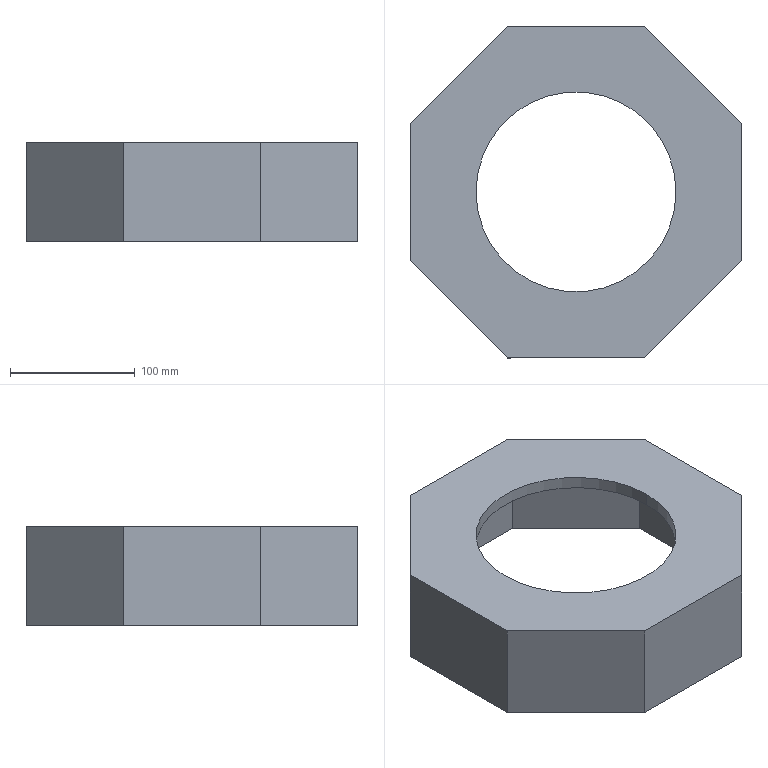Part | SolidWorks | features Cut 1, Extrusion 1, Shell 1 | 1 solid | 21 faces | box 265.563 x 265.563 x 80 mm | volume 975982 mm3 | plane 19 | cylinder 2 | commonest cylinder face diameters 160 x2
STEP:
#1=CARTESIAN_POINT('',(-679.884,-90.,70.));
#2=VERTEX_POINT('',#1);
#3=CARTESIAN_POINT('',(-519.884,-90.,70.));
#4=VERTEX_POINT('',#3);
#5=CARTESIAN_POINT('',(-599.884,-90.,70.));
#6=DIRECTION('',(0.,0.,1.));
#7=DIRECTION('',(1.,0.,0.));
#8=AXIS2_PLACEMENT_3D('',#5,#6,#7);
#9=CIRCLE('',#8,80.);
#10=EDGE_CURVE('',#2,#4,#9,.T.);
#11=ORIENTED_EDGE('',*,*,#10,.F.);
#12=CARTESIAN_POINT('',(-679.884,-90.,80.));
#13=VERTEX_POINT('',#12);
#14=CARTESIAN_POINT('',(-679.884,-90.,0.));
#15=DIRECTION('',(0.,0.,1.));
#16=VECTOR('',#15,1000.);
#17=LINE('',#14,#16);
#18=EDGE_CURVE('',#2,#13,#17,.T.);
#19=ORIENTED_EDGE('',*,*,#18,.T.);
#20=CARTESIAN_POINT('',(-519.884,-90.,80.));
#21=VERTEX_POINT('',#20);
#22=CARTESIAN_POINT('',(-599.884,-90.,80.));
#23=DIRECTION('',(0.,0.,1.));
#24=DIRECTION('',(1.,0.,0.));
#25=AXIS2_PLACEMENT_3D('',#22,#23,#24);
#26=CIRCLE('',#25,80.);
#27=EDGE_CURVE('',#13,#21,#26,.T.);
#28=ORIENTED_EDGE('',*,*,#27,.T.);
#29=CARTESIAN_POINT('',(-519.884,-90.,0.));
#30=DIRECTION('',(0.,0.,1.));
#31=VECTOR('',#30,1000.);
#32=LINE('',#29,#31);
#33=EDGE_CURVE('',#4,#21,#32,.T.);
#34=ORIENTED_EDGE('',*,*,#33,.F.);
#35=EDGE_LOOP('',(#11,#19,#28,#34));
#36=FACE_OUTER_BOUND('',#35,.T.);
#37=CARTESIAN_POINT('',(-599.884,-90.,0.));
#38=DIRECTION('',(0.,0.,1.));
#39=DIRECTION('',(1.,0.,0.));
#40=AXIS2_PLACEMENT_3D('',#37,#38,#39);
#41=CYLINDRICAL_SURFACE('',#40,80.);
#42=ADVANCED_FACE('',(#36),#41,.F.);
#43=CARTESIAN_POINT('',(-467.102,-145.,0.));
#44=VERTEX_POINT('',#43);
#45=CARTESIAN_POINT('',(-467.102,-35.,0.));
#46=VERTEX_POINT('',#45);
#47=CARTESIAN_POINT('',(-467.102,-145.,0.));
#48=DIRECTION('',(0.,1.,0.));
#49=VECTOR('',#48,1000.);
#50=LINE('',#47,#49);
#51=EDGE_CURVE('',#44,#46,#50,.T.);
#52=ORIENTED_EDGE('',*,*,#51,.T.);
#53=CARTESIAN_POINT('',(-467.102,-35.,80.));
#54=VERTEX_POINT('',#53);
#55=CARTESIAN_POINT('',(-467.102,-35.,80.));
#56=DIRECTION('',(0.,0.,-1.));
#57=VECTOR('',#56,1000.);
#58=LINE('',#55,#57);
#59=EDGE_CURVE('',#54,#46,#58,.T.);
#60=ORIENTED_EDGE('',*,*,#59,.F.);
#61=CARTESIAN_POINT('',(-467.102,-145.,80.));
#62=VERTEX_POINT('',#61);
#63=CARTESIAN_POINT('',(-467.102,-145.,80.));
#64=DIRECTION('',(0.,1.,0.));
#65=VECTOR('',#64,1000.);
#66=LINE('',#63,#65);
#67=EDGE_CURVE('',#62,#54,#66,.T.);
#68=ORIENTED_EDGE('',*,*,#67,.F.);
#69=CARTESIAN_POINT('',(-467.102,-145.,80.));
#70=DIRECTION('',(0.,0.,-1.));
#71=VECTOR('',#70,1000.);
#72=LINE('',#69,#71);
#73=EDGE_CURVE('',#62,#44,#72,.T.);
#74=ORIENTED_EDGE('',*,*,#73,.T.);
#75=EDGE_LOOP('',(#52,#60,#68,#74));
#76=FACE_OUTER_BOUND('',#75,.T.);
#77=CARTESIAN_POINT('',(-467.102,-145.,80.));
#78=DIRECTION('',(-1.,0.,0.));
#79=DIRECTION('',(0.,-1.,0.));
#80=AXIS2_PLACEMENT_3D('',#77,#78,#79);
#81=PLANE('',#80);
#82=ADVANCED_FACE('',(#76),#81,.F.);
#83=CARTESIAN_POINT('',(-544.884,42.782,0.));
#84=VERTEX_POINT('',#83);
#85=CARTESIAN_POINT('',(-467.102,-35.,0.));
#86=DIRECTION('',(-0.7071,0.7071,0.));
#87=VECTOR('',#86,1000.);
#88=LINE('',#85,#87);
#89=EDGE_CURVE('',#46,#84,#88,.T.);
#90=ORIENTED_EDGE('',*,*,#89,.T.);
#91=CARTESIAN_POINT('',(-544.884,42.782,80.));
#92=VERTEX_POINT('',#91);
#93=CARTESIAN_POINT('',(-544.884,42.782,80.));
#94=DIRECTION('',(0.,0.,-1.));
#95=VECTOR('',#94,1000.);
#96=LINE('',#93,#95);
#97=EDGE_CURVE('',#92,#84,#96,.T.);
#98=ORIENTED_EDGE('',*,*,#97,.F.);
#99=CARTESIAN_POINT('',(-467.102,-35.,80.));
#100=DIRECTION('',(-0.7071,0.7071,0.));
#101=VECTOR('',#100,1000.);
#102=LINE('',#99,#101);
#103=EDGE_CURVE('',#54,#92,#102,.T.);
#104=ORIENTED_EDGE('',*,*,#103,.F.);
#105=ORIENTED_EDGE('',*,*,#59,.T.);
#106=EDGE_LOOP('',(#90,#98,#104,#105));
#107=FACE_OUTER_BOUND('',#106,.T.);
#108=CARTESIAN_POINT('',(-467.102,-35.,80.));
#109=DIRECTION('',(-0.7071,-0.7071,0.));
#110=DIRECTION('',(0.7071,-0.7071,0.));
#111=AXIS2_PLACEMENT_3D('',#108,#109,#110);
#112=PLANE('',#111);
#113=ADVANCED_FACE('',(#107),#112,.F.);
#114=CARTESIAN_POINT('',(-654.884,42.782,0.));
#115=VERTEX_POINT('',#114);
#116=CARTESIAN_POINT('',(-544.884,42.782,0.));
#117=DIRECTION('',(-1.,0.,0.));
#118=VECTOR('',#117,1000.);
#119=LINE('',#116,#118);
#120=EDGE_CURVE('',#84,#115,#119,.T.);
#121=ORIENTED_EDGE('',*,*,#120,.T.);
#122=CARTESIAN_POINT('',(-654.884,42.782,80.));
#123=VERTEX_POINT('',#122);
#124=CARTESIAN_POINT('',(-654.884,42.782,80.));
#125=DIRECTION('',(0.,0.,-1.));
#126=VECTOR('',#125,1000.);
#127=LINE('',#124,#126);
#128=EDGE_CURVE('',#123,#115,#127,.T.);
#129=ORIENTED_EDGE('',*,*,#128,.F.);
#130=CARTESIAN_POINT('',(-544.884,42.782,80.));
#131=DIRECTION('',(-1.,0.,0.));
#132=VECTOR('',#131,1000.);
#133=LINE('',#130,#132);
#134=EDGE_CURVE('',#92,#123,#133,.T.);
#135=ORIENTED_EDGE('',*,*,#134,.F.);
#136=ORIENTED_EDGE('',*,*,#97,.T.);
#137=EDGE_LOOP('',(#121,#129,#135,#136));
#138=FACE_OUTER_BOUND('',#137,.T.);
#139=CARTESIAN_POINT('',(-544.884,42.782,80.));
#140=DIRECTION('',(0.,-1.,0.));
#141=DIRECTION('',(1.,0.,0.));
#142=AXIS2_PLACEMENT_3D('',#139,#140,#141);
#143=PLANE('',#142);
#144=ADVANCED_FACE('',(#138),#143,.F.);
#145=CARTESIAN_POINT('',(-732.666,-35.,0.));
#146=VERTEX_POINT('',#145);
#147=CARTESIAN_POINT('',(-654.884,42.782,0.));
#148=DIRECTION('',(-0.7071,-0.7071,0.));
#149=VECTOR('',#148,1000.);
#150=LINE('',#147,#149);
#151=EDGE_CURVE('',#115,#146,#150,.T.);
#152=ORIENTED_EDGE('',*,*,#151,.T.);
#153=CARTESIAN_POINT('',(-732.666,-35.,80.));
#154=VERTEX_POINT('',#153);
#155=CARTESIAN_POINT('',(-732.666,-35.,80.));
#156=DIRECTION('',(0.,0.,-1.));
#157=VECTOR('',#156,1000.);
#158=LINE('',#155,#157);
#159=EDGE_CURVE('',#154,#146,#158,.T.);
#160=ORIENTED_EDGE('',*,*,#159,.F.);
#161=CARTESIAN_POINT('',(-654.884,42.782,80.));
#162=DIRECTION('',(-0.7071,-0.7071,0.));
#163=VECTOR('',#162,1000.);
#164=LINE('',#161,#163);
#165=EDGE_CURVE('',#123,#154,#164,.T.);
#166=ORIENTED_EDGE('',*,*,#165,.F.);
#167=ORIENTED_EDGE('',*,*,#128,.T.);
#168=EDGE_LOOP('',(#152,#160,#166,#167));
#169=FACE_OUTER_BOUND('',#168,.T.);
#170=CARTESIAN_POINT('',(-654.884,42.782,80.));
#171=DIRECTION('',(0.7071,-0.7071,0.));
#172=DIRECTION('',(0.7071,0.7071,0.));
#173=AXIS2_PLACEMENT_3D('',#170,#171,#172);
#174=PLANE('',#173);
#175=ADVANCED_FACE('',(#169),#174,.F.);
#176=CARTESIAN_POINT('',(-732.666,-145.,0.));
#177=VERTEX_POINT('',#176);
#178=CARTESIAN_POINT('',(-732.666,-35.,0.));
#179=DIRECTION('',(0.,-1.,0.));
#180=VECTOR('',#179,1000.);
#181=LINE('',#178,#180);
#182=EDGE_CURVE('',#146,#177,#181,.T.);
#183=ORIENTED_EDGE('',*,*,#182,.T.);
#184=CARTESIAN_POINT('',(-732.666,-145.,80.));
#185=VERTEX_POINT('',#184);
#186=CARTESIAN_POINT('',(-732.666,-145.,80.));
#187=DIRECTION('',(0.,0.,-1.));
#188=VECTOR('',#187,1000.);
#189=LINE('',#186,#188);
#190=EDGE_CURVE('',#185,#177,#189,.T.);
#191=ORIENTED_EDGE('',*,*,#190,.F.);
#192=CARTESIAN_POINT('',(-732.666,-35.,80.));
#193=DIRECTION('',(0.,-1.,0.));
#194=VECTOR('',#193,1000.);
#195=LINE('',#192,#194);
#196=EDGE_CURVE('',#154,#185,#195,.T.);
#197=ORIENTED_EDGE('',*,*,#196,.F.);
#198=ORIENTED_EDGE('',*,*,#159,.T.);
#199=EDGE_LOOP('',(#183,#191,#197,#198));
#200=FACE_OUTER_BOUND('',#199,.T.);
#201=CARTESIAN_POINT('',(-732.666,-35.,80.));
#202=DIRECTION('',(1.,0.,0.));
#203=DIRECTION('',(0.,1.,0.));
#204=AXIS2_PLACEMENT_3D('',#201,#202,#203);
#205=PLANE('',#204);
#206=ADVANCED_FACE('',(#200),#205,.F.);
#207=CARTESIAN_POINT('',(-654.884,-222.782,0.));
#208=VERTEX_POINT('',#207);
#209=CARTESIAN_POINT('',(-732.666,-145.,0.));
#210=DIRECTION('',(0.7071,-0.7071,0.));
#211=VECTOR('',#210,1000.);
#212=LINE('',#209,#211);
#213=EDGE_CURVE('',#177,#208,#212,.T.);
#214=ORIENTED_EDGE('',*,*,#213,.T.);
#215=CARTESIAN_POINT('',(-654.884,-222.782,80.));
#216=VERTEX_POINT('',#215);
#217=CARTESIAN_POINT('',(-654.884,-222.782,80.));
#218=DIRECTION('',(0.,0.,-1.));
#219=VECTOR('',#218,1000.);
#220=LINE('',#217,#219);
#221=EDGE_CURVE('',#216,#208,#220,.T.);
#222=ORIENTED_EDGE('',*,*,#221,.F.);
#223=CARTESIAN_POINT('',(-732.666,-145.,80.));
#224=DIRECTION('',(0.7071,-0.7071,0.));
#225=VECTOR('',#224,1000.);
#226=LINE('',#223,#225);
#227=EDGE_CURVE('',#185,#216,#226,.T.);
#228=ORIENTED_EDGE('',*,*,#227,.F.);
#229=ORIENTED_EDGE('',*,*,#190,.T.);
#230=EDGE_LOOP('',(#214,#222,#228,#229));
#231=FACE_OUTER_BOUND('',#230,.T.);
#232=CARTESIAN_POINT('',(-732.666,-145.,80.));
#233=DIRECTION('',(0.7071,0.7071,0.));
#234=DIRECTION('',(-0.7071,0.7071,0.));
#235=AXIS2_PLACEMENT_3D('',#232,#233,#234);
#236=PLANE('',#235);
#237=ADVANCED_FACE('',(#231),#236,.F.);
#238=CARTESIAN_POINT('',(-544.884,-222.782,0.));
#239=VERTEX_POINT('',#238);
#240=CARTESIAN_POINT('',(-654.884,-222.782,0.));
#241=DIRECTION('',(1.,0.,0.));
#242=VECTOR('',#241,1000.);
#243=LINE('',#240,#242);
#244=EDGE_CURVE('',#208,#239,#243,.T.);
#245=ORIENTED_EDGE('',*,*,#244,.T.);
#246=CARTESIAN_POINT('',(-544.884,-222.782,80.));
#247=VERTEX_POINT('',#246);
#248=CARTESIAN_POINT('',(-544.884,-222.782,80.));
#249=DIRECTION('',(0.,0.,-1.));
#250=VECTOR('',#249,1000.);
#251=LINE('',#248,#250);
#252=EDGE_CURVE('',#247,#239,#251,.T.);
#253=ORIENTED_EDGE('',*,*,#252,.F.);
#254=CARTESIAN_POINT('',(-654.884,-222.782,80.));
#255=DIRECTION('',(1.,0.,0.));
#256=VECTOR('',#255,1000.);
#257=LINE('',#254,#256);
#258=EDGE_CURVE('',#216,#247,#257,.T.);
#259=ORIENTED_EDGE('',*,*,#258,.F.);
#260=ORIENTED_EDGE('',*,*,#221,.T.);
#261=EDGE_LOOP('',(#245,#253,#259,#260));
#262=FACE_OUTER_BOUND('',#261,.T.);
#263=CARTESIAN_POINT('',(-654.884,-222.782,80.));
#264=DIRECTION('',(0.,1.,0.));
#265=DIRECTION('',(-1.,0.,0.));
#266=AXIS2_PLACEMENT_3D('',#263,#264,#265);
#267=PLANE('',#266);
#268=ADVANCED_FACE('',(#262),#267,.F.);
#269=CARTESIAN_POINT('',(-544.884,-222.782,0.));
#270=DIRECTION('',(0.7071,0.7071,0.));
#271=VECTOR('',#270,1000.);
#272=LINE('',#269,#271);
#273=EDGE_CURVE('',#239,#44,#272,.T.);
#274=ORIENTED_EDGE('',*,*,#273,.T.);
#275=ORIENTED_EDGE('',*,*,#73,.F.);
#276=CARTESIAN_POINT('',(-544.884,-222.782,80.));
#277=DIRECTION('',(0.7071,0.7071,0.));
#278=VECTOR('',#277,1000.);
#279=LINE('',#276,#278);
#280=EDGE_CURVE('',#247,#62,#279,.T.);
#281=ORIENTED_EDGE('',*,*,#280,.F.);
#282=ORIENTED_EDGE('',*,*,#252,.T.);
#283=EDGE_LOOP('',(#274,#275,#281,#282));
#284=FACE_OUTER_BOUND('',#283,.T.);
#285=CARTESIAN_POINT('',(-544.884,-222.782,80.));
#286=DIRECTION('',(-0.7071,0.7071,0.));
#287=DIRECTION('',(-0.7071,-0.7071,0.));
#288=AXIS2_PLACEMENT_3D('',#285,#286,#287);
#289=PLANE('',#288);
#290=ADVANCED_FACE('',(#284),#289,.F.);
#291=CARTESIAN_POINT('',(-599.884,-90.,80.));
#292=DIRECTION('',(0.,0.,1.));
#293=DIRECTION('',(1.,0.,0.));
#294=AXIS2_PLACEMENT_3D('',#291,#292,#293);
#295=CIRCLE('',#294,80.);
#296=EDGE_CURVE('',#21,#13,#295,.T.);
#297=ORIENTED_EDGE('',*,*,#296,.F.);
#298=ORIENTED_EDGE('',*,*,#27,.F.);
#299=EDGE_LOOP('',(#297,#298));
#300=FACE_BOUND('',#299,.T.);
#301=ORIENTED_EDGE('',*,*,#67,.T.);
#302=ORIENTED_EDGE('',*,*,#103,.T.);
#303=ORIENTED_EDGE('',*,*,#134,.T.);
#304=ORIENTED_EDGE('',*,*,#165,.T.);
#305=ORIENTED_EDGE('',*,*,#196,.T.);
#306=ORIENTED_EDGE('',*,*,#227,.T.);
#307=ORIENTED_EDGE('',*,*,#258,.T.);
#308=ORIENTED_EDGE('',*,*,#280,.T.);
#309=EDGE_LOOP('',(#301,#302,#303,#304,#305,#306,#307,#308));
#310=FACE_OUTER_BOUND('',#309,.T.);
#311=CARTESIAN_POINT('',(0.,0.,80.));
#312=DIRECTION('',(0.,0.,1.));
#313=DIRECTION('',(1.,0.,0.));
#314=AXIS2_PLACEMENT_3D('',#311,#312,#313);
#315=PLANE('',#314);
#316=ADVANCED_FACE('',(#300,#310),#315,.T.);
#317=CARTESIAN_POINT('',(-549.026,-212.782,0.));
#318=VERTEX_POINT('',#317);
#319=CARTESIAN_POINT('',(-477.102,-140.858,0.));
#320=VERTEX_POINT('',#319);
#321=CARTESIAN_POINT('',(-551.955,-215.711,0.));
#322=DIRECTION('',(0.7071,0.7071,0.));
#323=VECTOR('',#322,1000.);
#324=LINE('',#321,#323);
#325=EDGE_CURVE('',#318,#320,#324,.T.);
#326=ORIENTED_EDGE('',*,*,#325,.T.);
#327=CARTESIAN_POINT('',(-477.102,-39.142,0.));
#328=VERTEX_POINT('',#327);
#329=CARTESIAN_POINT('',(-477.102,-145.,0.));
#330=DIRECTION('',(0.,1.,0.));
#331=VECTOR('',#330,1000.);
#332=LINE('',#329,#331);
#333=EDGE_CURVE('',#320,#328,#332,.T.);
#334=ORIENTED_EDGE('',*,*,#333,.T.);
#335=CARTESIAN_POINT('',(-549.026,32.782,0.));
#336=VERTEX_POINT('',#335);
#337=CARTESIAN_POINT('',(-474.174,-42.071,0.));
#338=DIRECTION('',(-0.7071,0.7071,0.));
#339=VECTOR('',#338,1000.);
#340=LINE('',#337,#339);
#341=EDGE_CURVE('',#328,#336,#340,.T.);
#342=ORIENTED_EDGE('',*,*,#341,.T.);
#343=CARTESIAN_POINT('',(-650.742,32.782,0.));
#344=VERTEX_POINT('',#343);
#345=CARTESIAN_POINT('',(-544.884,32.782,0.));
#346=DIRECTION('',(-1.,0.,0.));
#347=VECTOR('',#346,1000.);
#348=LINE('',#345,#347);
#349=EDGE_CURVE('',#336,#344,#348,.T.);
#350=ORIENTED_EDGE('',*,*,#349,.T.);
#351=CARTESIAN_POINT('',(-722.666,-39.142,0.));
#352=VERTEX_POINT('',#351);
#353=CARTESIAN_POINT('',(-647.813,35.711,0.));
#354=DIRECTION('',(-0.7071,-0.7071,0.));
#355=VECTOR('',#354,1000.);
#356=LINE('',#353,#355);
#357=EDGE_CURVE('',#344,#352,#356,.T.);
#358=ORIENTED_EDGE('',*,*,#357,.T.);
#359=CARTESIAN_POINT('',(-722.666,-140.858,0.));
#360=VERTEX_POINT('',#359);
#361=CARTESIAN_POINT('',(-722.666,-35.,0.));
#362=DIRECTION('',(0.,-1.,0.));
#363=VECTOR('',#362,1000.);
#364=LINE('',#361,#363);
#365=EDGE_CURVE('',#352,#360,#364,.T.);
#366=ORIENTED_EDGE('',*,*,#365,.T.);
#367=CARTESIAN_POINT('',(-650.742,-212.782,0.));
#368=VERTEX_POINT('',#367);
#369=CARTESIAN_POINT('',(-725.595,-137.929,0.));
#370=DIRECTION('',(0.7071,-0.7071,0.));
#371=VECTOR('',#370,1000.);
#372=LINE('',#369,#371);
#373=EDGE_CURVE('',#360,#368,#372,.T.);
#374=ORIENTED_EDGE('',*,*,#373,.T.);
#375=CARTESIAN_POINT('',(-654.884,-212.782,0.));
#376=DIRECTION('',(1.,0.,0.));
#377=VECTOR('',#376,1000.);
#378=LINE('',#375,#377);
#379=EDGE_CURVE('',#368,#318,#378,.T.);
#380=ORIENTED_EDGE('',*,*,#379,.T.);
#381=EDGE_LOOP('',(#326,#334,#342,#350,#358,#366,#374,#380));
#382=FACE_BOUND('',#381,.T.);
#383=ORIENTED_EDGE('',*,*,#51,.F.);
#384=ORIENTED_EDGE('',*,*,#273,.F.);
#385=ORIENTED_EDGE('',*,*,#244,.F.);
#386=ORIENTED_EDGE('',*,*,#213,.F.);
#387=ORIENTED_EDGE('',*,*,#182,.F.);
#388=ORIENTED_EDGE('',*,*,#151,.F.);
#389=ORIENTED_EDGE('',*,*,#120,.F.);
#390=ORIENTED_EDGE('',*,*,#89,.F.);
#391=EDGE_LOOP('',(#383,#384,#385,#386,#387,#388,#389,#390));
#392=FACE_OUTER_BOUND('',#391,.T.);
#393=CARTESIAN_POINT('',(0.,0.,0.));
#394=DIRECTION('',(0.,0.,1.));
#395=DIRECTION('',(1.,0.,0.));
#396=AXIS2_PLACEMENT_3D('',#393,#394,#395);
#397=PLANE('',#396);
#398=ADVANCED_FACE('',(#382,#392),#397,.F.);
#399=ORIENTED_EDGE('',*,*,#333,.F.);
#400=CARTESIAN_POINT('',(-477.102,-140.858,70.));
#401=VERTEX_POINT('',#400);
#402=CARTESIAN_POINT('',(-477.102,-140.858,80.));
#403=DIRECTION('',(0.,0.,-1.));
#404=VECTOR('',#403,1000.);
#405=LINE('',#402,#404);
#406=EDGE_CURVE('',#401,#320,#405,.T.);
#407=ORIENTED_EDGE('',*,*,#406,.F.);
#408=CARTESIAN_POINT('',(-477.102,-39.142,70.));
#409=VERTEX_POINT('',#408);
#410=CARTESIAN_POINT('',(-477.102,-145.,70.));
#411=DIRECTION('',(0.,1.,0.));
#412=VECTOR('',#411,1000.);
#413=LINE('',#410,#412);
#414=EDGE_CURVE('',#401,#409,#413,.T.);
#415=ORIENTED_EDGE('',*,*,#414,.T.);
#416=CARTESIAN_POINT('',(-477.102,-39.142,80.));
#417=DIRECTION('',(0.,0.,-1.));
#418=VECTOR('',#417,1000.);
#419=LINE('',#416,#418);
#420=EDGE_CURVE('',#409,#328,#419,.T.);
#421=ORIENTED_EDGE('',*,*,#420,.T.);
#422=EDGE_LOOP('',(#399,#407,#415,#421));
#423=FACE_OUTER_BOUND('',#422,.T.);
#424=CARTESIAN_POINT('',(-477.102,-145.,80.));
#425=DIRECTION('',(-1.,0.,0.));
#426=DIRECTION('',(0.,-1.,0.));
#427=AXIS2_PLACEMENT_3D('',#424,#425,#426);
#428=PLANE('',#427);
#429=ADVANCED_FACE('',(#423),#428,.T.);
#430=ORIENTED_EDGE('',*,*,#341,.F.);
#431=ORIENTED_EDGE('',*,*,#420,.F.);
#432=CARTESIAN_POINT('',(-549.026,32.782,70.));
#433=VERTEX_POINT('',#432);
#434=CARTESIAN_POINT('',(-474.174,-42.071,70.));
#435=DIRECTION('',(-0.7071,0.7071,0.));
#436=VECTOR('',#435,1000.);
#437=LINE('',#434,#436);
#438=EDGE_CURVE('',#409,#433,#437,.T.);
#439=ORIENTED_EDGE('',*,*,#438,.T.);
#440=CARTESIAN_POINT('',(-549.026,32.782,80.));
#441=DIRECTION('',(0.,0.,-1.));
#442=VECTOR('',#441,1000.);
#443=LINE('',#440,#442);
#444=EDGE_CURVE('',#433,#336,#443,.T.);
#445=ORIENTED_EDGE('',*,*,#444,.T.);
#446=EDGE_LOOP('',(#430,#431,#439,#445));
#447=FACE_OUTER_BOUND('',#446,.T.);
#448=CARTESIAN_POINT('',(-474.174,-42.071,80.));
#449=DIRECTION('',(-0.7071,-0.7071,0.));
#450=DIRECTION('',(0.7071,-0.7071,0.));
#451=AXIS2_PLACEMENT_3D('',#448,#449,#450);
#452=PLANE('',#451);
#453=ADVANCED_FACE('',(#447),#452,.T.);
#454=ORIENTED_EDGE('',*,*,#349,.F.);
#455=ORIENTED_EDGE('',*,*,#444,.F.);
#456=CARTESIAN_POINT('',(-650.742,32.782,70.));
#457=VERTEX_POINT('',#456);
#458=CARTESIAN_POINT('',(-544.884,32.782,70.));
#459=DIRECTION('',(-1.,0.,0.));
#460=VECTOR('',#459,1000.);
#461=LINE('',#458,#460);
#462=EDGE_CURVE('',#433,#457,#461,.T.);
#463=ORIENTED_EDGE('',*,*,#462,.T.);
#464=CARTESIAN_POINT('',(-650.742,32.782,80.));
#465=DIRECTION('',(0.,0.,-1.));
#466=VECTOR('',#465,1000.);
#467=LINE('',#464,#466);
#468=EDGE_CURVE('',#457,#344,#467,.T.);
#469=ORIENTED_EDGE('',*,*,#468,.T.);
#470=EDGE_LOOP('',(#454,#455,#463,#469));
#471=FACE_OUTER_BOUND('',#470,.T.);
#472=CARTESIAN_POINT('',(-544.884,32.782,80.));
#473=DIRECTION('',(0.,-1.,0.));
#474=DIRECTION('',(1.,0.,0.));
#475=AXIS2_PLACEMENT_3D('',#472,#473,#474);
#476=PLANE('',#475);
#477=ADVANCED_FACE('',(#471),#476,.T.);
#478=ORIENTED_EDGE('',*,*,#357,.F.);
#479=ORIENTED_EDGE('',*,*,#468,.F.);
#480=CARTESIAN_POINT('',(-722.666,-39.142,70.));
#481=VERTEX_POINT('',#480);
#482=CARTESIAN_POINT('',(-647.813,35.711,70.));
#483=DIRECTION('',(-0.7071,-0.7071,0.));
#484=VECTOR('',#483,1000.);
#485=LINE('',#482,#484);
#486=EDGE_CURVE('',#457,#481,#485,.T.);
#487=ORIENTED_EDGE('',*,*,#486,.T.);
#488=CARTESIAN_POINT('',(-722.666,-39.142,80.));
#489=DIRECTION('',(0.,0.,-1.));
#490=VECTOR('',#489,1000.);
#491=LINE('',#488,#490);
#492=EDGE_CURVE('',#481,#352,#491,.T.);
#493=ORIENTED_EDGE('',*,*,#492,.T.);
#494=EDGE_LOOP('',(#478,#479,#487,#493));
#495=FACE_OUTER_BOUND('',#494,.T.);
#496=CARTESIAN_POINT('',(-647.813,35.711,80.));
#497=DIRECTION('',(0.7071,-0.7071,0.));
#498=DIRECTION('',(0.7071,0.7071,0.));
#499=AXIS2_PLACEMENT_3D('',#496,#497,#498);
#500=PLANE('',#499);
#501=ADVANCED_FACE('',(#495),#500,.T.);
#502=ORIENTED_EDGE('',*,*,#365,.F.);
#503=ORIENTED_EDGE('',*,*,#492,.F.);
#504=CARTESIAN_POINT('',(-722.666,-140.858,70.));
#505=VERTEX_POINT('',#504);
#506=CARTESIAN_POINT('',(-722.666,-35.,70.));
#507=DIRECTION('',(0.,-1.,0.));
#508=VECTOR('',#507,1000.);
#509=LINE('',#506,#508);
#510=EDGE_CURVE('',#481,#505,#509,.T.);
#511=ORIENTED_EDGE('',*,*,#510,.T.);
#512=CARTESIAN_POINT('',(-722.666,-140.858,80.));
#513=DIRECTION('',(0.,0.,-1.));
#514=VECTOR('',#513,1000.);
#515=LINE('',#512,#514);
#516=EDGE_CURVE('',#505,#360,#515,.T.);
#517=ORIENTED_EDGE('',*,*,#516,.T.);
#518=EDGE_LOOP('',(#502,#503,#511,#517));
#519=FACE_OUTER_BOUND('',#518,.T.);
#520=CARTESIAN_POINT('',(-722.666,-35.,80.));
#521=DIRECTION('',(1.,0.,0.));
#522=DIRECTION('',(0.,1.,0.));
#523=AXIS2_PLACEMENT_3D('',#520,#521,#522);
#524=PLANE('',#523);
#525=ADVANCED_FACE('',(#519),#524,.T.);
#526=ORIENTED_EDGE('',*,*,#373,.F.);
#527=ORIENTED_EDGE('',*,*,#516,.F.);
#528=CARTESIAN_POINT('',(-650.742,-212.782,70.));
#529=VERTEX_POINT('',#528);
#530=CARTESIAN_POINT('',(-725.595,-137.929,70.));
#531=DIRECTION('',(0.7071,-0.7071,0.));
#532=VECTOR('',#531,1000.);
#533=LINE('',#530,#532);
#534=EDGE_CURVE('',#505,#529,#533,.T.);
#535=ORIENTED_EDGE('',*,*,#534,.T.);
#536=CARTESIAN_POINT('',(-650.742,-212.782,80.));
#537=DIRECTION('',(0.,0.,-1.));
#538=VECTOR('',#537,1000.);
#539=LINE('',#536,#538);
#540=EDGE_CURVE('',#529,#368,#539,.T.);
#541=ORIENTED_EDGE('',*,*,#540,.T.);
#542=EDGE_LOOP('',(#526,#527,#535,#541));
#543=FACE_OUTER_BOUND('',#542,.T.);
#544=CARTESIAN_POINT('',(-725.595,-137.929,80.));
#545=DIRECTION('',(0.7071,0.7071,0.));
#546=DIRECTION('',(-0.7071,0.7071,0.));
#547=AXIS2_PLACEMENT_3D('',#544,#545,#546);
#548=PLANE('',#547);
#549=ADVANCED_FACE('',(#543),#548,.T.);
#550=ORIENTED_EDGE('',*,*,#379,.F.);
#551=ORIENTED_EDGE('',*,*,#540,.F.);
#552=CARTESIAN_POINT('',(-549.026,-212.782,70.));
#553=VERTEX_POINT('',#552);
#554=CARTESIAN_POINT('',(-654.884,-212.782,70.));
#555=DIRECTION('',(1.,0.,0.));
#556=VECTOR('',#555,1000.);
#557=LINE('',#554,#556);
#558=EDGE_CURVE('',#529,#553,#557,.T.);
#559=ORIENTED_EDGE('',*,*,#558,.T.);
#560=CARTESIAN_POINT('',(-549.026,-212.782,80.));
#561=DIRECTION('',(0.,0.,-1.));
#562=VECTOR('',#561,1000.);
#563=LINE('',#560,#562);
#564=EDGE_CURVE('',#553,#318,#563,.T.);
#565=ORIENTED_EDGE('',*,*,#564,.T.);
#566=EDGE_LOOP('',(#550,#551,#559,#565));
#567=FACE_OUTER_BOUND('',#566,.T.);
#568=CARTESIAN_POINT('',(-654.884,-212.782,80.));
#569=DIRECTION('',(0.,1.,0.));
#570=DIRECTION('',(-1.,0.,0.));
#571=AXIS2_PLACEMENT_3D('',#568,#569,#570);
#572=PLANE('',#571);
#573=ADVANCED_FACE('',(#567),#572,.T.);
#574=ORIENTED_EDGE('',*,*,#325,.F.);
#575=ORIENTED_EDGE('',*,*,#564,.F.);
#576=CARTESIAN_POINT('',(-551.955,-215.711,70.));
#577=DIRECTION('',(0.7071,0.7071,0.));
#578=VECTOR('',#577,1000.);
#579=LINE('',#576,#578);
#580=EDGE_CURVE('',#553,#401,#579,.T.);
#581=ORIENTED_EDGE('',*,*,#580,.T.);
#582=ORIENTED_EDGE('',*,*,#406,.T.);
#583=EDGE_LOOP('',(#574,#575,#581,#582));
#584=FACE_OUTER_BOUND('',#583,.T.);
#585=CARTESIAN_POINT('',(-551.955,-215.711,80.));
#586=DIRECTION('',(-0.7071,0.7071,0.));
#587=DIRECTION('',(-0.7071,-0.7071,0.));
#588=AXIS2_PLACEMENT_3D('',#585,#586,#587);
#589=PLANE('',#588);
#590=ADVANCED_FACE('',(#584),#589,.T.);
#591=CARTESIAN_POINT('',(-599.884,-90.,70.));
#592=DIRECTION('',(0.,0.,1.));
#593=DIRECTION('',(1.,0.,0.));
#594=AXIS2_PLACEMENT_3D('',#591,#592,#593);
#595=CIRCLE('',#594,80.);
#596=EDGE_CURVE('',#4,#2,#595,.T.);
#597=ORIENTED_EDGE('',*,*,#596,.T.);
#598=ORIENTED_EDGE('',*,*,#10,.T.);
#599=EDGE_LOOP('',(#597,#598));
#600=FACE_BOUND('',#599,.T.);
#601=ORIENTED_EDGE('',*,*,#414,.F.);
#602=ORIENTED_EDGE('',*,*,#580,.F.);
#603=ORIENTED_EDGE('',*,*,#558,.F.);
#604=ORIENTED_EDGE('',*,*,#534,.F.);
#605=ORIENTED_EDGE('',*,*,#510,.F.);
#606=ORIENTED_EDGE('',*,*,#486,.F.);
#607=ORIENTED_EDGE('',*,*,#462,.F.);
#608=ORIENTED_EDGE('',*,*,#438,.F.);
#609=EDGE_LOOP('',(#601,#602,#603,#604,#605,#606,#607,#608));
#610=FACE_OUTER_BOUND('',#609,.T.);
#611=CARTESIAN_POINT('',(0.,0.,70.));
#612=DIRECTION('',(0.,0.,1.));
#613=DIRECTION('',(1.,0.,0.));
#614=AXIS2_PLACEMENT_3D('',#611,#612,#613);
#615=PLANE('',#614);
#616=ADVANCED_FACE('',(#600,#610),#615,.F.);
#617=ORIENTED_EDGE('',*,*,#18,.F.);
#618=ORIENTED_EDGE('',*,*,#596,.F.);
#619=ORIENTED_EDGE('',*,*,#33,.T.);
#620=ORIENTED_EDGE('',*,*,#296,.T.);
#621=EDGE_LOOP('',(#617,#618,#619,#620));
#622=FACE_OUTER_BOUND('',#621,.T.);
#623=CARTESIAN_POINT('',(-599.884,-90.,0.));
#624=DIRECTION('',(0.,0.,1.));
#625=DIRECTION('',(1.,0.,0.));
#626=AXIS2_PLACEMENT_3D('',#623,#624,#625);
#627=CYLINDRICAL_SURFACE('',#626,80.);
#628=ADVANCED_FACE('',(#622),#627,.F.);
#629=CLOSED_SHELL('',(#42,#82,#113,#144,#175,#206,#237,#268,#290,#316,#398,#429,#453,#477,#501,#525,#549,#573,#590,#616,#628));
#630=MANIFOLD_SOLID_BREP('',#629);
#631=CARTESIAN_POINT('',(0.,0.,0.));
#632=DIRECTION('',(0.,0.,1.));
#633=DIRECTION('',(1.,0.,0.));
#634=AXIS2_PLACEMENT_3D('',#631,#632,#633);
#635=(LENGTH_UNIT()NAMED_UNIT(*)SI_UNIT(.MILLI.,.METRE.));
#636=UNCERTAINTY_MEASURE_WITH_UNIT(LENGTH_MEASURE(0.00001),#635,'','');
#637=(NAMED_UNIT(*)PLANE_ANGLE_UNIT()SI_UNIT($,.RADIAN.));
#638=(NAMED_UNIT(*)SI_UNIT($,.STERADIAN.)SOLID_ANGLE_UNIT());
#639=(GEOMETRIC_REPRESENTATION_CONTEXT(3)GLOBAL_UNCERTAINTY_ASSIGNED_CONTEXT((#636))GLOBAL_UNIT_ASSIGNED_CONTEXT((#635,#637,#638))REPRESENTATION_CONTEXT('',''));
#640=ADVANCED_BREP_SHAPE_REPRESENTATION('',(#630,#634),#639);